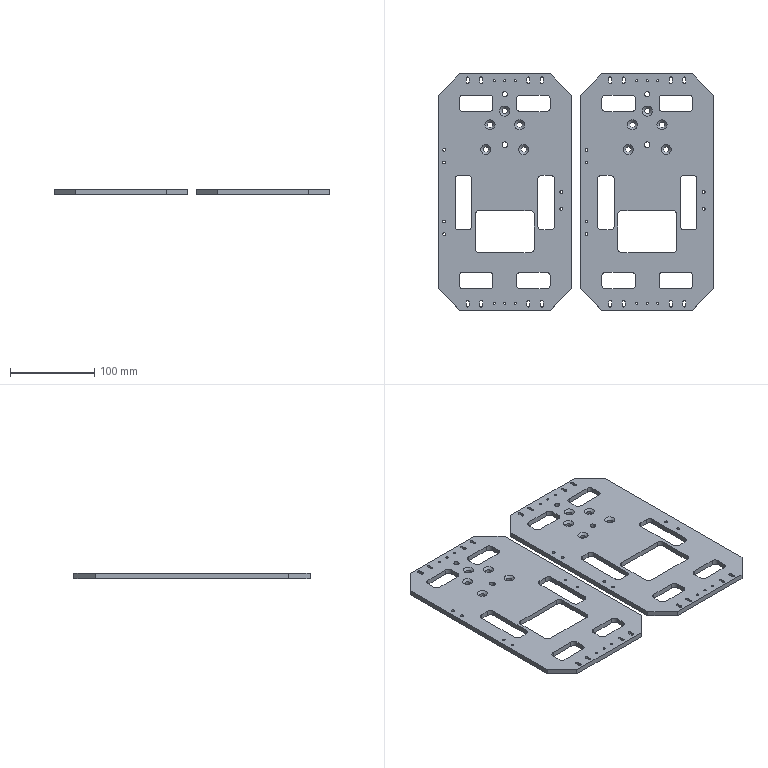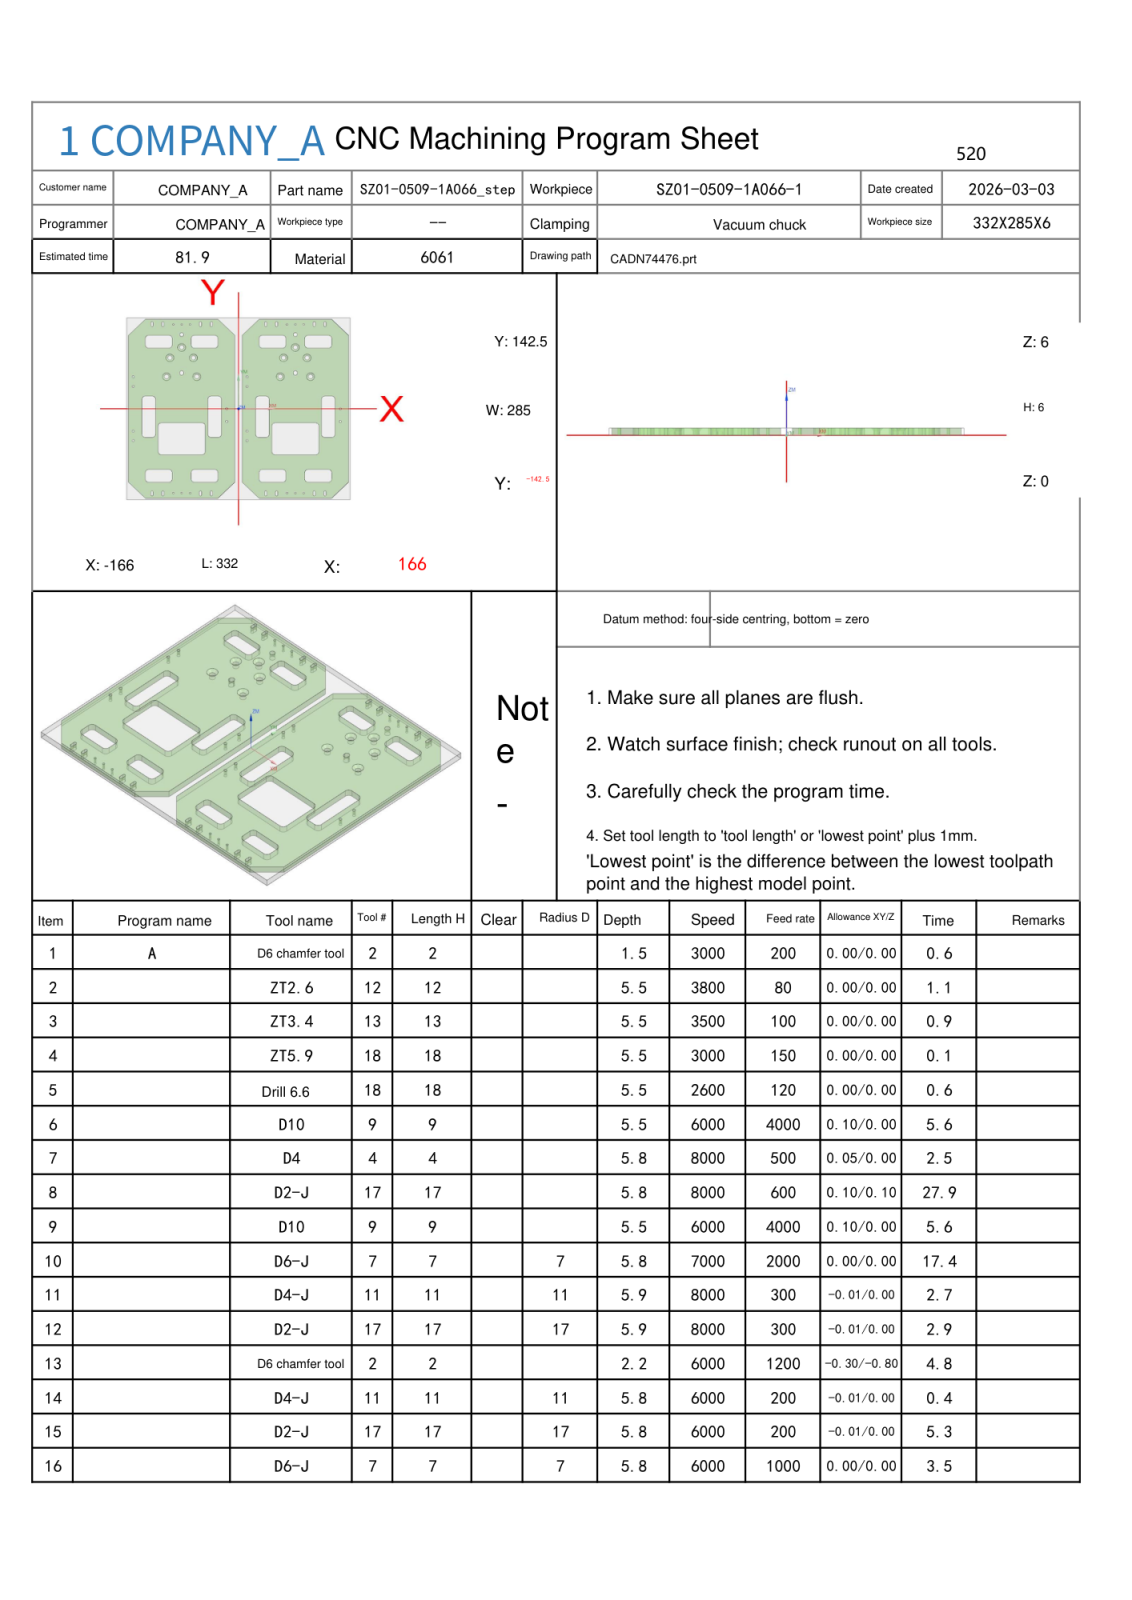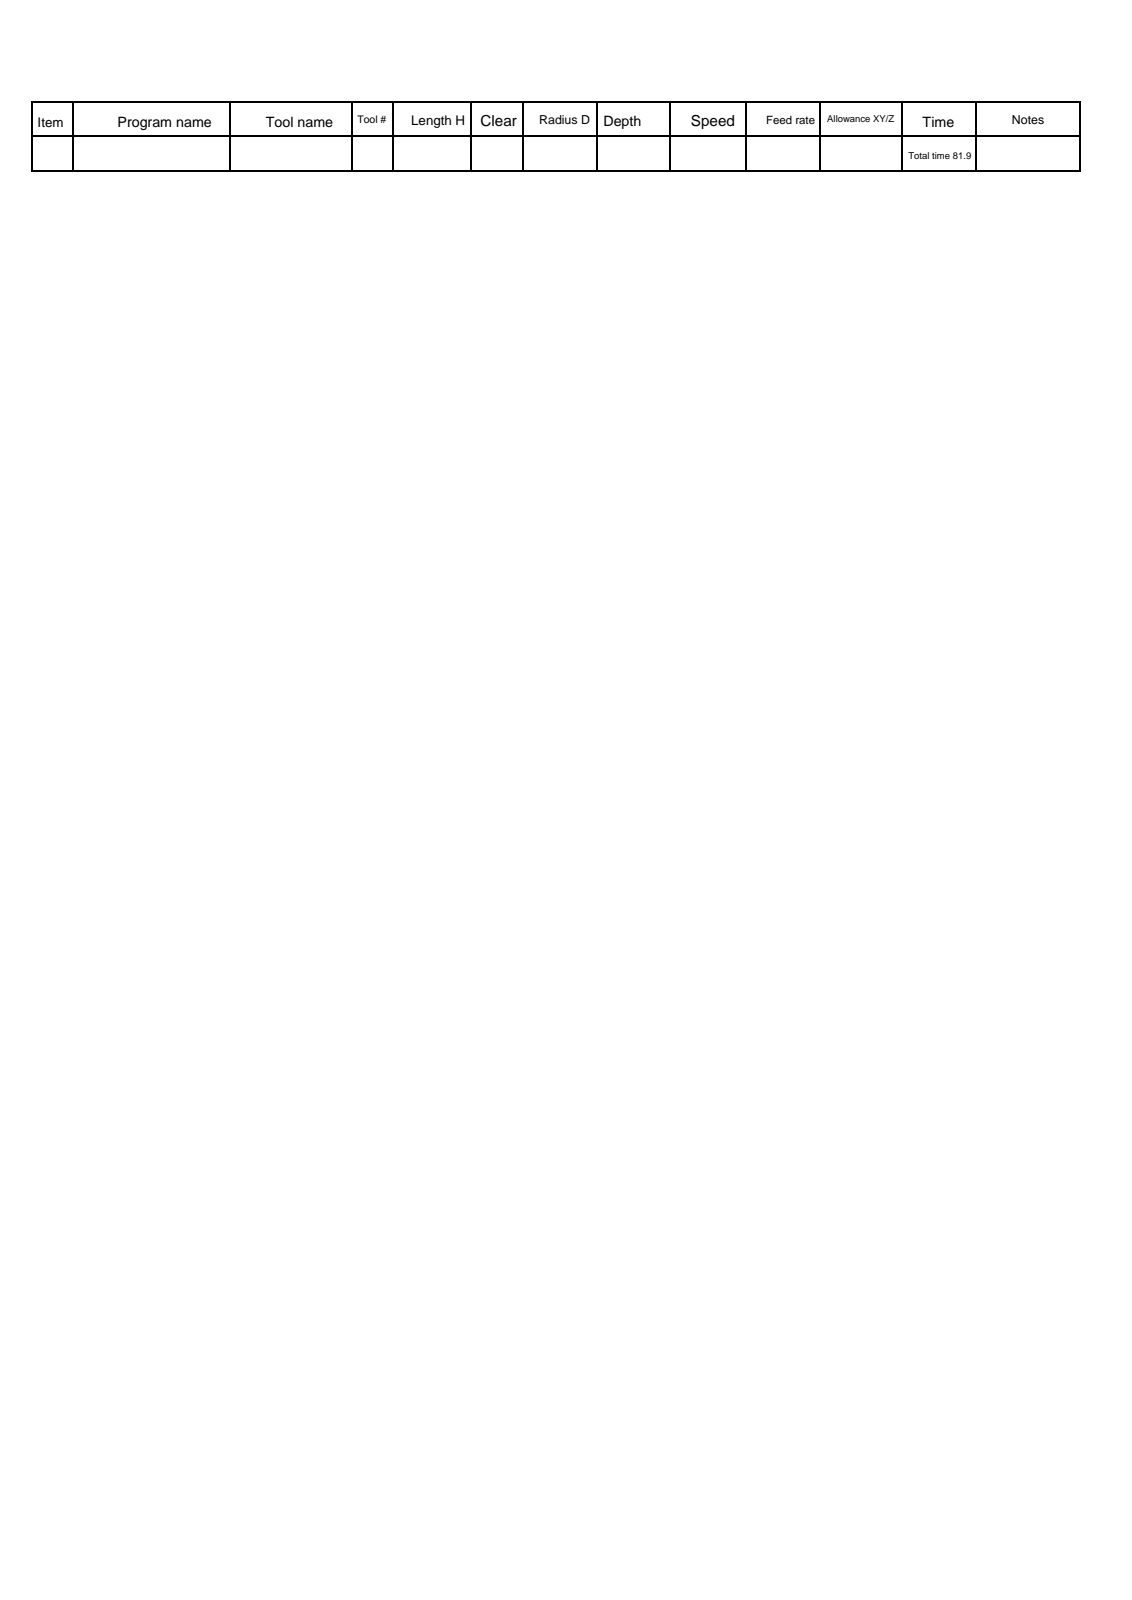NC program | NX | posted by the shop | part box 327 x 280 x 6 mm
Lines 10363 to 11471 of 31860:
N10 T07 M06
(D6-J  D=6. R=0. H=07 ce=0.00 di=0.00)
G00 G90 G54 X53.5 Y-66.801 M03 S6000
G43 H07 Z36.
M08
Z1.
G01 Z.5 F1000.
G41 D07
Y-68.
G03 X54.5 Y-69. I1. J0.0
G01 X114.5
G03 X116.5 Y-67. I0.0 J2.
G01 Y-27.
G03 X114.5 Y-25. I-2. J0.0
G01 X54.5
G03 X52.5 Y-27. I0.0 J-2.
G01 Y-67.
G03 X54.5 Y-69. I2. J0.0
G01 X55.
G03 X56. Y-68. I0.0 J1.
G01 G40 Y-67.8
Z1.
G00 Z36.
X-115.5 Y-66.801
Z1.
G01 Z.5
G41 D07
Y-68.
G03 X-114.5 Y-69. I1. J0.0
G01 X-54.5
G03 X-52.5 Y-67. I0.0 J2.
G01 Y-27.
G03 X-54.5 Y-25. I-2. J0.0
G01 X-114.5
G03 X-116.5 Y-27. I0.0 J-2.
G01 Y-67.
G03 X-114.5 Y-69. I2. J0.0
G01 X-114.
G03 X-113. Y-68. I0.0 J1.
G01 G40 Y-67.8
Z1.
G00 Z36.
G00 G90 X138.3 Y-41. M03 S6000
Z36.
Z1.
G01 Z.5 F1000.
G41 D07
X139.5
G03 X140.5 Y-40. I0.0 J1.
G01 Y15.
G03 X138.5 Y17. I-2. J0.0
G01 X128.5
G03 X126.5 Y15. I0.0 J-2.
G01 Y-40.
G03 X128.5 Y-42. I2. J0.0
G01 X138.5
G03 X140.5 Y-40. I0.0 J2.
G01 Y-39.5
G03 X139.5 Y-38.5 I-1. J0.0
G01 G40 X139.3
Z1.
G00 Z36.
X40.301 Y-41.
Z1.
G01 Z.5
G41 D07
X41.5
G03 X42.5 Y-40. I0.0 J1.
G01 Y15.
G03 X40.5 Y17. I-2. J0.0
G01 X30.5
G03 X28.5 Y15. I0.0 J-2.
G01 Y-40.
G03 X30.5 Y-42. I2. J0.0
G01 X40.5
G03 X42.5 Y-40. I0.0 J2.
G01 Y-39.5
G03 X41.5 Y-38.5 I-1. J0.0
G01 G40 X41.3
Z1.
G00 Z36.
X-40.301 Y16.
Z1.
G01 Z.5
G41 D07
X-41.5
G03 X-42.5 Y15. I0.0 J-1.
G01 Y-40.
G03 X-40.5 Y-42. I2. J0.0
G01 X-30.5
G03 X-28.5 Y-40. I0.0 J2.
G01 Y15.
G03 X-30.5 Y17. I-2. J0.0
G01 X-40.5
G03 X-42.5 Y15. I0.0 J-2.
G01 Y14.5
G03 X-41.5 Y13.5 I1. J0.0
G01 G40 X-41.3
Z1.
G00 Z36.
X-138.301 Y16.
Z1.
G01 Z.5
G41 D07
X-139.5
G03 X-140.5 Y15. I0.0 J-1.
G01 Y-40.
G03 X-138.5 Y-42. I2. J0.0
G01 X-128.5
G03 X-126.5 Y-40. I0.0 J2.
G01 Y15.
G03 X-128.5 Y17. I-2. J0.0
G01 X-138.5
G03 X-140.5 Y15. I0.0 J-2.
G01 Y14.5
G03 X-139.5 Y13.5 I1. J0.0
G01 G40 X-139.3
Z1.
G00 Z36.
G00 G90 X-102.5 Y109.8 M03 S6000
Z36.
Z1.
G01 Z.5 F1000.
G41 D07
Y111.
G03 X-103.5 Y112. I-1. J0.0
G01 X-133.5
G03 X-135.5 Y110. I0.0 J-2.
G01 Y100.
G03 X-133.5 Y98. I2. J0.0
G01 X-103.5
G03 X-101.5 Y100. I0.0 J2.
G01 Y110.
G03 X-103.5 Y112. I-2. J0.0
G01 X-104.
G03 X-105. Y111. I0.0 J-1.
G01 G40 Y110.8
Z1.
G00 Z36.
X-34.5 Y109.8
Z1.
G01 Z.5
G41 D07
Y111.
G03 X-35.5 Y112. I-1. J0.0
G01 X-65.5
G03 X-67.5 Y110. I0.0 J-2.
G01 Y100.
G03 X-65.5 Y98. I2. J0.0
G01 X-35.5
G03 X-33.5 Y100. I0.0 J2.
G01 Y110.
G03 X-35.5 Y112. I-2. J0.0
G01 X-36.
G03 X-37. Y111. I0.0 J-1.
G01 G40 Y110.8
Z1.
G00 Z36.
X66.5 Y109.8
Z1.
G01 Z.5
G41 D07
Y111.
G03 X65.5 Y112. I-1. J0.0
G01 X35.5
G03 X33.5 Y110. I0.0 J-2.
G01 Y100.
G03 X35.5 Y98. I2. J0.0
G01 X65.5
G03 X67.5 Y100. I0.0 J2.
G01 Y110.
G03 X65.5 Y112. I-2. J0.0
G01 X65.
G03 X64. Y111. I0.0 J-1.
G01 G40 Y110.8
Z1.
G00 Z36.
X134.5 Y109.8
Z1.
G01 Z.5
G41 D07
Y111.
G03 X133.5 Y112. I-1. J0.0
G01 X103.5
G03 X101.5 Y110. I0.0 J-2.
G01 Y100.
G03 X103.5 Y98. I2. J0.0
G01 X133.5
G03 X135.5 Y100. I0.0 J2.
G01 Y110.
G03 X133.5 Y112. I-2. J0.0
G01 X133.
G03 X132. Y111. I0.0 J-1.
G01 G40 Y110.8
Z1.
G00 Z36.
X102.5 Y-109.8
Z1.
G01 Z.5
G41 D07
Y-111.
G03 X103.5 Y-112. I1. J0.0
G01 X133.5
G03 X135.5 Y-110. I0.0 J2.
G01 Y-100.
G03 X133.5 Y-98. I-2. J0.0
G01 X103.5
G03 X101.5 Y-100. I0.0 J-2.
G01 Y-110.
G03 X103.5 Y-112. I2. J0.0
G01 X104.
G03 X105. Y-111. I0.0 J1.
G01 G40 Y-110.8
Z1.
G00 Z36.
X34.793 Y-110.707
Z1.
G01 Z.5
G41 D07
X34.5 Y-111.
G03 X35.5 Y-112. I1. J0.0
G01 X65.5
G03 X67.5 Y-110. I0.0 J2.
G01 Y-100.
G03 X65.5 Y-98. I-2. J0.0
G01 X35.5
G03 X33.5 Y-100. I0.0 J-2.
G01 Y-110.
G03 X35.5 Y-112. I2. J0.0
G01 X36.
G03 X37. Y-111. I0.0 J1.
G01 G40 Y-110.8
Z1.
G00 Z36.
X-66.5 Y-109.8
Z1.
G01 Z.5
G41 D07
Y-111.
G03 X-65.5 Y-112. I1. J0.0
G01 X-35.5
G03 X-33.5 Y-110. I0.0 J2.
G01 Y-100.
G03 X-35.5 Y-98. I-2. J0.0
G01 X-65.5
G03 X-67.5 Y-100. I0.0 J-2.
G01 Y-110.
G03 X-65.5 Y-112. I2. J0.0
G01 X-65.
G03 X-64. Y-111. I0.0 J1.
G01 G40 Y-110.8
Z1.
G00 Z36.
X-134.5 Y-109.8
Z1.
G01 Z.5
G41 D07
Y-111.
G03 X-133.5 Y-112. I1. J0.0
G01 X-103.5
G03 X-101.5 Y-110. I0.0 J2.
G01 Y-100.
G03 X-103.5 Y-98. I-2. J0.0
G01 X-133.5
G03 X-135.5 Y-100. I0.0 J-2.
G01 Y-110.
G03 X-133.5 Y-112. I2. J0.0
G01 X-133.
G03 X-132. Y-111. I0.0 J1.
G01 G40 Y-110.8
Z1.
G00 Z36.
G00 G90 X53.5 Y-66.901 M03 S6000
Z36.
Z.7
G01 Z.2 F1000.
G41 D07
Y-68.
G03 X54.5 Y-69. I1. J0.0
G01 X114.5
G03 X116.5 Y-67. I0.0 J2.
G01 Y-27.
G03 X114.5 Y-25. I-2. J0.0
G01 X54.5
G03 X52.5 Y-27. I0.0 J-2.
G01 Y-67.
G03 X54.5 Y-69. I2. J0.0
G01 X55.
G03 X56. Y-68. I0.0 J1.
G01 G40 Y-67.9
Z.7
G00 Z36.
X-115.5 Y-66.9
Z.7
G01 Z.2
G41 D07
Y-68.
G03 X-114.5 Y-69. I1. J0.0
G01 X-54.5
G03 X-52.5 Y-67. I0.0 J2.
G01 Y-27.
G03 X-54.5 Y-25. I-2. J0.0
G01 X-114.5
G03 X-116.5 Y-27. I0.0 J-2.
G01 Y-67.
G03 X-114.5 Y-69. I2. J0.0
G01 X-114.
G03 X-113. Y-68. I0.0 J1.
G01 G40 Y-67.9
Z.7
G00 Z36.
G00 G90 X138.401 Y-41. M03 S6000
Z36.
Z.7
G01 Z.2 F1000.
G41 D07
X139.5
G03 X140.5 Y-40. I0.0 J1.
G01 Y15.
G03 X138.5 Y17. I-2. J0.0
G01 X128.5
G03 X126.5 Y15. I0.0 J-2.
G01 Y-40.
G03 X128.5 Y-42. I2. J0.0
G01 X138.5
G03 X140.5 Y-40. I0.0 J2.
G01 Y-39.5
G03 X139.5 Y-38.5 I-1. J0.0
G01 G40 X139.4
Z.7
G00 Z36.
X40.4 Y-41.
Z.7
G01 Z.2
G41 D07
X41.5
G03 X42.5 Y-40. I0.0 J1.
G01 Y15.
G03 X40.5 Y17. I-2. J0.0
G01 X30.5
G03 X28.5 Y15. I0.0 J-2.
G01 Y-40.
G03 X30.5 Y-42. I2. J0.0
G01 X40.5
G03 X42.5 Y-40. I0.0 J2.
G01 Y-39.5
G03 X41.5 Y-38.5 I-1. J0.0
G01 G40 X41.4
Z.7
G00 Z36.
X-40.401 Y16.
Z.7
G01 Z.2
G41 D07
X-41.5
G03 X-42.5 Y15. I0.0 J-1.
G01 Y-40.
G03 X-40.5 Y-42. I2. J0.0
G01 X-30.5
G03 X-28.5 Y-40. I0.0 J2.
G01 Y15.
G03 X-30.5 Y17. I-2. J0.0
G01 X-40.5
G03 X-42.5 Y15. I0.0 J-2.
G01 Y14.5
G03 X-41.5 Y13.5 I1. J0.0
G01 G40 X-41.4
Z.7
G00 Z36.
X-138.4 Y16.
Z.7
G01 Z.2
G41 D07
X-139.5
G03 X-140.5 Y15. I0.0 J-1.
G01 Y-40.
G03 X-138.5 Y-42. I2. J0.0
G01 X-128.5
G03 X-126.5 Y-40. I0.0 J2.
G01 Y15.
G03 X-128.5 Y17. I-2. J0.0
G01 X-138.5
G03 X-140.5 Y15. I0.0 J-2.
G01 Y14.5
G03 X-139.5 Y13.5 I1. J0.0
G01 G40 X-139.4
Z.7
G00 Z36.
G00 G90 X-102.793 Y110.707 M03 S6000
Z36.
Z.7
G01 Z.2 F1000.
G41 D07
X-102.5 Y111.
G03 X-103.5 Y112. I-1. J0.0
G01 X-133.5
G03 X-135.5 Y110. I0.0 J-2.
G01 Y100.
G03 X-133.5 Y98. I2. J0.0
G01 X-103.5
G03 X-101.5 Y100. I0.0 J2.
G01 Y110.
G03 X-103.5 Y112. I-2. J0.0
G01 X-104.
G03 X-105. Y111. I0.0 J-1.
G01 G40 Y110.9
Z.7
G00 Z36.
X-34.5 Y109.9
Z.7
G01 Z.2
G41 D07
Y111.
G03 X-35.5 Y112. I-1. J0.0
G01 X-65.5
G03 X-67.5 Y110. I0.0 J-2.
G01 Y100.
G03 X-65.5 Y98. I2. J0.0
G01 X-35.5
G03 X-33.5 Y100. I0.0 J2.
G01 Y110.
G03 X-35.5 Y112. I-2. J0.0
G01 X-36.
G03 X-37. Y111. I0.0 J-1.
G01 G40 Y110.9
Z.7
G00 Z36.
X66.5 Y109.9
Z.7
G01 Z.2
G41 D07
Y111.
G03 X65.5 Y112. I-1. J0.0
G01 X35.5
G03 X33.5 Y110. I0.0 J-2.
G01 Y100.
G03 X35.5 Y98. I2. J0.0
G01 X65.5
G03 X67.5 Y100. I0.0 J2.
G01 Y110.
G03 X65.5 Y112. I-2. J0.0
G01 X65.
G03 X64. Y111. I0.0 J-1.
G01 G40 Y110.9
Z.7
G00 Z36.
X134.5 Y109.9
Z.7
G01 Z.2
G41 D07
Y111.
G03 X133.5 Y112. I-1. J0.0
G01 X103.5
G03 X101.5 Y110. I0.0 J-2.
G01 Y100.
G03 X103.5 Y98. I2. J0.0
G01 X133.5
G03 X135.5 Y100. I0.0 J2.
G01 Y110.
G03 X133.5 Y112. I-2. J0.0
G01 X133.
G03 X132. Y111. I0.0 J-1.
G01 G40 Y110.9
Z.7
G00 Z36.
X102.5 Y-109.9
Z.7
G01 Z.2
G41 D07
Y-111.
G03 X103.5 Y-112. I1. J0.0
G01 X133.5
G03 X135.5 Y-110. I0.0 J2.
G01 Y-100.
G03 X133.5 Y-98. I-2. J0.0
G01 X103.5
G03 X101.5 Y-100. I0.0 J-2.
G01 Y-110.
G03 X103.5 Y-112. I2. J0.0
G01 X104.
G03 X105. Y-111. I0.0 J1.
G01 G40 Y-110.9
Z.7
G00 Z36.
X34.5 Y-109.901
Z.7
G01 Z.2
G41 D07
Y-111.
G03 X35.5 Y-112. I1. J0.0
G01 X65.5
G03 X67.5 Y-110. I0.0 J2.
G01 Y-100.
G03 X65.5 Y-98. I-2. J0.0
G01 X35.5
G03 X33.5 Y-100. I0.0 J-2.
G01 Y-110.
G03 X35.5 Y-112. I2. J0.0
G01 X36.
G03 X37. Y-111. I0.0 J1.
G01 G40 Y-110.9
Z.7
G00 Z36.
X-66.5 Y-109.9
Z.7
G01 Z.2
G41 D07
Y-111.
G03 X-65.5 Y-112. I1. J0.0
G01 X-35.5
G03 X-33.5 Y-110. I0.0 J2.
G01 Y-100.
G03 X-35.5 Y-98. I-2. J0.0
G01 X-65.5
G03 X-67.5 Y-100. I0.0 J-2.
G01 Y-110.
G03 X-65.5 Y-112. I2. J0.0
G01 X-65.
G03 X-64. Y-111. I0.0 J1.
G01 G40 Y-110.9
Z.7
G00 Z36.
X-134.5 Y-109.9
Z.7
G01 Z.2
G41 D07
Y-111.
G03 X-133.5 Y-112. I1. J0.0
G01 X-103.5
G03 X-101.5 Y-110. I0.0 J2.
G01 Y-100.
G03 X-103.5 Y-98. I-2. J0.0
G01 X-133.5
G03 X-135.5 Y-100. I0.0 J-2.
G01 Y-110.
G03 X-133.5 Y-112. I2. J0.0
G01 X-133.
G03 X-132. Y-111. I0.0 J1.
G01 G40 Y-110.9
Z.7
G00 Z36.
G00 G90 X-104.104 Y49.533 M03 S7000
Z36.
Z7.5
G01 X-104.1 Y49.546 Z7.499 F2000.
X-104.025 Y50.008 Z7.475
X-104.024 Y50.476 Z7.45
X-104.096 Y50.938 Z7.426
X-104.239 Y51.384 Z7.401
X-104.45 Y51.801 Z7.377
X-104.724 Y52.181 Z7.352
X-105.054 Y52.513 Z7.328
X-105.431 Y52.789 Z7.303
X-105.848 Y53.003 Z7.279
X-106.292 Y53.149 Z7.254
X-106.632 Y53.212 Z7.236
X-107.072 Y53.234 Z7.213
X-107.416 Y53.205 Z7.195
X-107.861 Y53.108 Z7.171
X-108.285 Y52.944 Z7.147
X-108.679 Y52.717 Z7.123
X-109.035 Y52.433 Z7.099
X-109.343 Y52.099 Z7.076
X-109.596 Y51.721 Z7.052
X-109.79 Y51.31 Z7.028
X-109.919 Y50.873 Z7.004
X-109.979 Y50.423 Z6.98
Y50.077 Z6.962
X-109.93 Y49.684 Z6.941
X-109.83 Y49.301 Z6.921
X-109.679 Y48.935 Z6.9
X-109.509 Y48.634 Z6.882
X-109.223 Y48.259 Z6.857
X-108.881 Y47.933 Z6.832
X-108.492 Y47.665 Z6.807
X-108.065 Y47.462 Z6.783
X-107.612 Y47.329 Z6.758
X-107.143 Y47.269 Z6.733
X-106.671 Y47.284 Z6.708
X-106.207 Y47.373 Z6.684
X-105.763 Y47.534 Z6.659
X-105.35 Y47.763 Z6.634
X-104.978 Y48.055 Z6.609
X-104.657 Y48.402 Z6.585
X-104.459 Y48.685 Z6.567
X-104.246 Y49.101 Z6.542
X-104.1 Y49.546 Z6.518
X-104.025 Y50.008 Z6.493
X-104.024 Y50.476 Z6.468
X-104.096 Y50.938 Z6.444
X-104.239 Y51.384 Z6.419
X-104.45 Y51.801 Z6.395
X-104.724 Y52.181 Z6.37
X-105.054 Y52.513 Z6.346
X-105.431 Y52.789 Z6.321
X-105.848 Y53.003 Z6.297
X-106.292 Y53.149 Z6.272
X-106.632 Y53.212 Z6.254
X-107.072 Y53.234 Z6.231
X-107.416 Y53.205 Z6.213
X-107.861 Y53.108 Z6.189
X-108.285 Y52.944 Z6.165
X-108.679 Y52.717 Z6.141
X-109.035 Y52.433 Z6.118
X-109.343 Y52.099 Z6.094
X-109.596 Y51.721 Z6.07
X-109.79 Y51.31 Z6.046
X-109.919 Y50.873 Z6.022
X-109.979 Y50.423 Z5.998
Y50.25 Z5.989
G03 X-107. Y47.271 I2.979 J0.0
X-104.021 Y50.25 I0.0 J2.979
X-107. Y53.229 I-2.979 J0.0
X-109.979 Y50.25 I0.0 J-2.979
G01 X-109.973 Y50.19 Z5.984
X-109.966 Y50.129 Z5.979
G03 X-107. Y47.281 I2.966 J.121
X-104.031 Y50.25 I0.0 J2.969
X-107. Y53.219 I-2.969 J0.0
X-109.969 Y50.25 I0.0 J-2.969
G01 X-109.963 Y50.19 Z5.973
X-109.956 Y50.129 Z5.968
G03 X-107. Y47.292 I2.956 J.121
X-104.042 Y50.25 I0.0 J2.958
X-107. Y53.208 I-2.958 J0.0
X-109.958 Y50.25 I0.0 J-2.958
G01 X-109.952 Y50.19 Z5.963
X-109.945 Y50.129 Z5.958
G03 X-107. Y47.302 I2.945 J.121
X-104.052 Y50.25 I0.0 J2.948
X-107. Y53.198 I-2.948 J0.0
X-109.948 Y50.25 I0.0 J-2.948
G01 X-109.942 Y50.19 Z5.952
X-109.934 Y50.129 Z5.947
G03 X-107. Y47.313 I2.934 J.121
X-104.063 Y50.25 I0.0 J2.937
X-107. Y53.187 I-2.937 J0.0
X-109.937 Y50.25 I0.0 J-2.937
G01 X-109.931 Y50.19 Z5.942
X-109.924 Y50.129 Z5.936
G03 X-107. Y47.324 I2.924 J.121
X-104.074 Y50.25 I0.0 J2.926
X-107. Y53.176 I-2.926 J0.0
X-109.926 Y50.25 I0.0 J-2.926
G01 X-109.92 Y50.19 Z5.931
X-109.913 Y50.129 Z5.926
G03 X-107. Y47.334 I2.913 J.121
X-104.084 Y50.25 I0.0 J2.916
X-107. Y53.166 I-2.916 J0.0
X-109.916 Y50.25 I0.0 J-2.916
G01 X-109.91 Y50.19 Z5.92
X-109.903 Y50.129 Z5.915
G03 X-107. Y47.345 I2.903 J.121
X-104.095 Y50.25 I0.0 J2.905
X-107. Y53.155 I-2.905 J0.0
X-109.905 Y50.25 I0.0 J-2.905
G01 X-109.899 Y50.19 Z5.91
X-109.892 Y50.129 Z5.905
G03 X-107. Y47.355 I2.892 J.121
X-104.105 Y50.25 I0.0 J2.895
X-107. Y53.145 I-2.895 J0.0
X-109.895 Y50.25 I0.0 J-2.895
G01 X-109.889 Y50.19 Z5.899
X-109.881 Y50.129 Z5.894
G03 X-107. Y47.366 I2.881 J.121
X-104.116 Y50.25 I0.0 J2.884
X-107. Y53.134 I-2.884 J0.0
X-109.884 Y50.25 I0.0 J-2.884
G01 X-109.878 Y50.19 Z5.889
X-109.871 Y50.129 Z5.883
G03 X-107. Y47.377 I2.871 J.121
X-104.127 Y50.25 I0.0 J2.873
X-107. Y53.123 I-2.873 J0.0
X-109.873 Y50.25 I0.0 J-2.873
G01 X-109.867 Y50.19 Z5.878
X-109.86 Y50.129 Z5.873
G03 X-107. Y47.387 I2.86 J.121
X-104.137 Y50.25 I0.0 J2.863
X-107. Y53.113 I-2.863 J0.0
X-109.863 Y50.25 I0.0 J-2.863
G01 X-109.857 Y50.19 Z5.867
X-109.85 Y50.129 Z5.862
G03 X-107. Y47.398 I2.85 J.121
X-104.148 Y50.25 I0.0 J2.852
X-107. Y53.102 I-2.852 J0.0
X-109.852 Y50.25 I0.0 J-2.852
G01 X-109.846 Y50.19 Z5.857
X-109.839 Y50.129 Z5.852
G03 X-107. Y47.408 I2.839 J.121
X-104.158 Y50.25 I0.0 J2.842
X-107. Y53.092 I-2.842 J0.0
X-109.842 Y50.25 I0.0 J-2.842
G01 X-109.836 Y50.19 Z5.846
X-109.828 Y50.129 Z5.841
G03 X-107. Y47.419 I2.828 J.121
X-104.169 Y50.25 I0.0 J2.831
X-107. Y53.081 I-2.831 J0.0
X-109.831 Y50.25 I0.0 J-2.831
G01 X-109.825 Y50.19 Z5.836
X-109.818 Y50.129 Z5.83
G03 X-107. Y47.43 I2.818 J.121
X-104.18 Y50.25 I0.0 J2.82
X-107. Y53.07 I-2.82 J0.0
X-109.82 Y50.25 I0.0 J-2.82
G01 X-109.814 Y50.19 Z5.825
X-109.807 Y50.129 Z5.82
G03 X-107. Y47.44 I2.807 J.121
X-104.19 Y50.25 I0.0 J2.81
X-107. Y53.06 I-2.81 J0.0
X-109.81 Y50.25 I0.0 J-2.81
G01 X-109.804 Y50.19 Z5.814
X-109.796 Y50.129 Z5.809
G03 X-107. Y47.451 I2.796 J.121
X-104.201 Y50.25 I0.0 J2.799
X-107. Y53.049 I-2.799 J0.0
X-109.799 Y50.25 I0.0 J-2.799
G01 X-109.793 Y50.19 Z5.804
X-109.786 Y50.129 Z5.798
G03 X-107. Y47.462 I2.786 J.121
X-104.212 Y50.25 I0.0 J2.788
X-107. Y53.038 I-2.788 J0.0
X-109.788 Y50.25 I0.0 J-2.788
G01 X-109.783 Y50.19 Z5.793
X-109.775 Y50.129 Z5.788
G03 X-107. Y47.472 I2.775 J.121
X-104.222 Y50.25 I0.0 J2.778
X-107. Y53.028 I-2.778 J0.0
X-109.778 Y50.25 I0.0 J-2.778
G01 X-109.772 Y50.19 Z5.783
X-109.765 Y50.129 Z5.777
G03 X-107. Y47.483 I2.765 J.121
X-104.233 Y50.25 I0.0 J2.767
X-107. Y53.017 I-2.767 J0.0
X-109.767 Y50.25 I0.0 J-2.767
G01 X-109.761 Y50.19 Z5.772
X-109.754 Y50.129 Z5.767
G03 X-107. Y47.493 I2.754 J.121
X-104.243 Y50.25 I0.0 J2.757
X-107. Y53.007 I-2.757 J0.0
X-109.757 Y50.25 I0.0 J-2.757
G01 X-109.751 Y50.19 Z5.761
X-109.743 Y50.129 Z5.756
G03 X-107. Y47.504 I2.743 J.121
X-104.254 Y50.25 I0.0 J2.746
X-107. Y52.996 I-2.746 J0.0
X-109.746 Y50.25 I0.0 J-2.746
G01 X-109.74 Y50.19 Z5.751
X-109.733 Y50.129 Z5.745
G03 X-107. Y47.515 I2.733 J.121
X-104.265 Y50.25 I0.0 J2.735
X-107. Y52.985 I-2.735 J0.0
X-109.735 Y50.25 I0.0 J-2.735
G01 X-109.729 Y50.19 Z5.74
X-109.722 Y50.129 Z5.735
G03 X-107. Y47.525 I2.722 J.121
X-104.275 Y50.25 I0.0 J2.725
X-107. Y52.975 I-2.725 J0.0
X-109.725 Y50.25 I0.0 J-2.725
G01 X-109.719 Y50.19 Z5.73
X-109.712 Y50.129 Z5.724
G03 X-107. Y47.536 I2.712 J.121
X-104.286 Y50.25 I0.0 J2.714
X-107. Y52.964 I-2.714 J0.0
X-109.714 Y50.25 I0.0 J-2.714
G01 X-109.708 Y50.19 Z5.719
X-109.701 Y50.129 Z5.714
G03 X-107. Y47.546 I2.701 J.121
X-104.296 Y50.25 I0.0 J2.704
X-107. Y52.954 I-2.704 J0.0
X-109.704 Y50.25 I0.0 J-2.704
G01 X-109.698 Y50.19 Z5.708
X-109.69 Y50.129 Z5.703
G03 X-107. Y47.557 I2.69 J.121
X-104.307 Y50.25 I0.0 J2.693
X-107. Y52.943 I-2.693 J0.0
X-109.693 Y50.25 I0.0 J-2.693
G01 X-109.687 Y50.19 Z5.698
X-109.68 Y50.129 Z5.692
G03 X-107. Y47.568 I2.68 J.121
X-104.318 Y50.25 I0.0 J2.682
X-107. Y52.932 I-2.682 J0.0
X-109.682 Y50.25 I0.0 J-2.682
G01 X-109.676 Y50.19 Z5.687
X-109.669 Y50.129 Z5.682
G03 X-107. Y47.578 I2.669 J.121
X-104.328 Y50.25 I0.0 J2.672
X-107. Y52.922 I-2.672 J0.0
X-109.672 Y50.25 I0.0 J-2.672
G01 X-109.666 Y50.19 Z5.676
X-109.658 Y50.129 Z5.671
G03 X-107. Y47.589 I2.658 J.121
X-104.339 Y50.25 I0.0 J2.661
X-107. Y52.911 I-2.661 J0.0
X-109.661 Y50.25 I0.0 J-2.661
G01 X-109.655 Y50.19 Z5.666
X-109.648 Y50.129 Z5.661
G03 X-107. Y47.599 I2.648 J.121
X-104.349 Y50.25 I0.0 J2.651
X-107. Y52.901 I-2.651 J0.0
X-109.651 Y50.25 I0.0 J-2.651
G01 X-109.645 Y50.19 Z5.655
X-109.637 Y50.129 Z5.65
G03 X-107. Y47.61 I2.637 J.121
X-104.36 Y50.25 I0.0 J2.64
X-107. Y52.89 I-2.64 J0.0
X-109.64 Y50.25 I0.0 J-2.64
G01 X-109.634 Y50.19 Z5.645
X-109.627 Y50.129 Z5.639
G03 X-107. Y47.621 I2.627 J.121
X-104.371 Y50.25 I0.0 J2.629
X-107. Y52.879 I-2.629 J0.0
X-109.629 Y50.25 I0.0 J-2.629
G01 X-109.623 Y50.19 Z5.634
X-109.616 Y50.129 Z5.629
G03 X-107. Y47.631 I2.616 J.121
X-104.381 Y50.25 I0.0 J2.619
X-107. Y52.869 I-2.619 J0.0
X-109.619 Y50.25 I0.0 J-2.619
G01 X-109.613 Y50.19 Z5.623
X-109.605 Y50.129 Z5.618
G03 X-107. Y47.642 I2.605 J.121
X-104.392 Y50.25 I0.0 J2.608
X-107. Y52.858 I-2.608 J0.0
X-109.608 Y50.25 I0.0 J-2.608
G01 X-109.602 Y50.19 Z5.613
X-109.595 Y50.129 Z5.608
G03 X-107. Y47.652 I2.595 J.121
X-104.402 Y50.25 I0.0 J2.598
X-107. Y52.848 I-2.598 J0.0
X-109.598 Y50.25 I0.0 J-2.598
G01 X-109.592 Y50.19 Z5.602
X-109.584 Y50.129 Z5.597
G03 X-107. Y47.663 I2.584 J.121
X-104.413 Y50.25 I0.0 J2.587
X-107. Y52.837 I-2.587 J0.0
X-109.587 Y50.25 I0.0 J-2.587
G01 X-109.581 Y50.19 Z5.592
X-109.574 Y50.129 Z5.586
G03 X-107. Y47.674 I2.574 J.121
X-104.424 Y50.25 I0.0 J2.576
X-107. Y52.826 I-2.576 J0.0
X-109.576 Y50.25 I0.0 J-2.576
G01 X-109.57 Y50.19 Z5.581
X-109.563 Y50.129 Z5.576
G03 X-107. Y47.684 I2.563 J.121
X-104.434 Y50.25 I0.0 J2.566
X-107. Y52.816 I-2.566 J0.0
X-109.566 Y50.25 I0.0 J-2.566
G01 X-109.56 Y50.19 Z5.57
X-109.552 Y50.129 Z5.565
G03 X-107. Y47.695 I2.552 J.121
X-104.445 Y50.25 I0.0 J2.555
X-107. Y52.805 I-2.555 J0.0
X-109.555 Y50.25 I0.0 J-2.555
G01 X-109.549 Y50.19 Z5.56
X-109.542 Y50.129 Z5.555
G03 X-107. Y47.705 I2.542 J.121
X-104.455 Y50.25 I0.0 J2.545
X-107. Y52.795 I-2.545 J0.0
X-109.545 Y50.25 I0.0 J-2.545
G01 X-109.539 Y50.19 Z5.549
X-109.531 Y50.129 Z5.544
G03 X-107. Y47.716 I2.531 J.121
X-104.466 Y50.25 I0.0 J2.534
X-107. Y52.784 I-2.534 J0.0
X-109.534 Y50.25 I0.0 J-2.534
G01 X-109.528 Y50.19 Z5.539
X-109.52 Y50.129 Z5.533
G03 X-107. Y47.727 I2.52 J.121
X-104.477 Y50.25 I0.0 J2.523
X-107. Y52.773 I-2.523 J0.0
X-109.523 Y50.25 I0.0 J-2.523
G01 X-109.517 Y50.19 Z5.528
X-109.51 Y50.129 Z5.523
G03 X-107. Y47.737 I2.51 J.121
X-104.487 Y50.25 I0.0 J2.513
X-107. Y52.763 I-2.513 J0.0
X-109.513 Y50.25 I0.0 J-2.513
G01 X-109.507 Y50.19 Z5.517
X-109.499 Y50.129 Z5.512
G03 X-107. Y47.748 I2.499 J.121
X-104.498 Y50.25 I0.0 J2.502
X-107. Y52.752 I-2.502 J0.0
X-109.502 Y50.25 I0.0 J-2.502
G01 X-109.496 Y50.19 Z5.507
X-109.489 Y50.129 Z5.501
G03 X-107. Y47.759 I2.489 J.121
X-104.509 Y50.25 I0.0 J2.491
X-107. Y52.741 I-2.491 J0.0
X-109.491 Y50.25 I0.0 J-2.491
G01 X-109.485 Y50.19 Z5.496
X-109.478 Y50.129 Z5.491
G03 X-107. Y47.769 I2.478 J.121
X-104.519 Y50.25 I0.0 J2.481
X-107. Y52.731 I-2.481 J0.0
X-109.481 Y50.25 I0.0 J-2.481
G01 X-109.475 Y50.19 Z5.486
X-109.467 Y50.129 Z5.48
G03 X-107. Y47.78 I2.467 J.121
X-104.53 Y50.25 I0.0 J2.47
X-107. Y52.72 I-2.47 J0.0
X-109.47 Y50.25 I0.0 J-2.47
G01 X-109.464 Y50.19 Z5.475
X-109.457 Y50.129 Z5.47
G03 X-107. Y47.79 I2.457 J.121
X-104.54 Y50.25 I0.0 J2.46
X-107. Y52.71 I-2.46 J0.0
X-109.46 Y50.25 I0.0 J-2.46
G01 X-109.454 Y50.19 Z5.464
X-109.446 Y50.129 Z5.459
G03 X-107. Y47.801 I2.446 J.121
X-104.551 Y50.25 I0.0 J2.449
X-107. Y52.699 I-2.449 J0.0
X-109.449 Y50.25 I0.0 J-2.449
G01 X-109.443 Y50.19 Z5.454
X-109.435 Y50.129 Z5.448
G03 X-107. Y47.812 I2.435 J.121
X-104.562 Y50.25 I0.0 J2.438
X-107. Y52.688 I-2.438 J0.0
X-109.438 Y50.25 I0.0 J-2.438
G01 X-109.432 Y50.19 Z5.443
X-109.425 Y50.129 Z5.438
G03 X-107. Y47.822 I2.425 J.121
X-104.572 Y50.25 I0.0 J2.428
X-107. Y52.678 I-2.428 J0.0
X-109.428 Y50.25 I0.0 J-2.428
G01 X-109.422 Y50.19 Z5.433
X-109.414 Y50.129 Z5.427
G03 X-107. Y47.833 I2.414 J.121
X-104.583 Y50.25 I0.0 J2.417
X-107. Y52.667 I-2.417 J0.0
X-109.417 Y50.25 I0.0 J-2.417
G01 X-109.411 Y50.19 Z5.422
X-109.404 Y50.129 Z5.417
G03 X-107. Y47.843 I2.404 J.121
X-104.593 Y50.25 I0.0 J2.407
X-107. Y52.657 I-2.407 J0.0
X-109.407 Y50.25 I0.0 J-2.407
G01 X-109.401 Y50.19 Z5.411
X-109.393 Y50.129 Z5.406
G03 X-107. Y47.854 I2.393 J.121
X-104.604 Y50.25 I0.0 J2.396
X-107. Y52.646 I-2.396 J0.0
X-109.396 Y50.25 I0.0 J-2.396
G01 X-109.39 Y50.19 Z5.401
X-109.382 Y50.129 Z5.395
G03 X-107. Y47.865 I2.382 J.121
X-104.615 Y50.25 I0.0 J2.385
X-107. Y52.635 I-2.385 J0.0
X-109.385 Y50.25 I0.0 J-2.385
G01 X-109.379 Y50.19 Z5.39
X-109.372 Y50.129 Z5.385
G03 X-107. Y47.875 I2.372 J.121
X-104.625 Y50.25 I0.0 J2.375
X-107. Y52.625 I-2.375 J0.0
X-109.375 Y50.25 I0.0 J-2.375
G01 X-109.369 Y50.19 Z5.38
X-109.361 Y50.129 Z5.374
G03 X-107. Y47.886 I2.361 J.121
X-104.636 Y50.25 I0.0 J2.364
X-107. Y52.614 I-2.364 J0.0
X-109.364 Y50.25 I0.0 J-2.364
G01 X-109.358 Y50.19 Z5.369
X-109.351 Y50.129 Z5.364
G03 X-107. Y47.896 I2.351 J.121
X-104.646 Y50.25 I0.0 J2.354
X-107. Y52.604 I-2.354 J0.0
X-109.354 Y50.25 I0.0 J-2.354
G01 X-109.348 Y50.19 Z5.358
X-109.34 Y50.129 Z5.353
G03 X-107. Y47.907 I2.34 J.121
X-104.657 Y50.25 I0.0 J2.343
X-107. Y52.593 I-2.343 J0.0
X-109.343 Y50.25 I0.0 J-2.343
G01 X-109.337 Y50.19 Z5.348
X-109.329 Y50.129 Z5.342
G03 X-107. Y47.918 I2.329 J.121
X-104.668 Y50.25 I0.0 J2.332
X-107. Y52.582 I-2.332 J0.0
X-109.332 Y50.25 I0.0 J-2.332
G01 X-109.326 Y50.19 Z5.337
X-109.319 Y50.129 Z5.332
G03 X-107. Y47.928 I2.319 J.121
X-104.678 Y50.25 I0.0 J2.322
X-107. Y52.572 I-2.322 J0.0
X-109.322 Y50.25 I0.0 J-2.322
G01 X-109.316 Y50.19 Z5.326
X-109.308 Y50.129 Z5.321
G03 X-107. Y47.939 I2.308 J.121
X-104.689 Y50.25 I0.0 J2.311
X-107. Y52.561 I-2.311 J0.0
X-109.311 Y50.25 I0.0 J-2.311
G01 X-109.305 Y50.19 Z5.316
X-109.297 Y50.129 Z5.311
G03 X-107. Y47.949 I2.297 J.121
X-104.699 Y50.25 I0.0 J2.301
X-107. Y52.551 I-2.301 J0.0
X-109.301 Y50.25 I0.0 J-2.301
G01 X-109.294 Y50.19 Z5.305
X-109.287 Y50.129 Z5.3
G03 X-107. Y47.96 I2.287 J.121
X-104.71 Y50.25 I0.0 J2.29
X-107. Y52.54 I-2.29 J0.0
X-109.29 Y50.25 I0.0 J-2.29
G01 X-109.284 Y50.19 Z5.295
X-109.276 Y50.129 Z5.289
G03 X-107. Y47.971 I2.276 J.121
X-104.721 Y50.25 I0.0 J2.279
X-107. Y52.529 I-2.279 J0.0
X-109.279 Y50.25 I0.0 J-2.279
G01 X-109.273 Y50.19 Z5.284
X-109.266 Y50.129 Z5.279
G03 X-107. Y47.981 I2.266 J.121
X-104.731 Y50.25 I0.0 J2.269
X-107. Y52.519 I-2.269 J0.0
X-109.269 Y50.25 I0.0 J-2.269
G01 X-109.263 Y50.19 Z5.273
X-109.255 Y50.129 Z5.268
G03 X-107. Y47.992 I2.255 J.121
X-104.742 Y50.25 I0.0 J2.258
X-107. Y52.508 I-2.258 J0.0
X-109.258 Y50.25 I0.0 J-2.258
G01 X-109.252 Y50.19 Z5.263
X-109.244 Y50.129 Z5.258
G03 X-107. Y48.002 I2.244 J.121
X-104.752 Y50.25 I0.0 J2.248
X-107. Y52.498 I-2.248 J0.0
X-109.248 Y50.25 I0.0 J-2.248
G01 X-109.241 Y50.19 Z5.252
X-109.234 Y50.129 Z5.247
G03 X-107. Y48.013 I2.234 J.121
X-104.763 Y50.25 I0.0 J2.237
X-107. Y52.487 I-2.237 J0.0
X-109.237 Y50.25 I0.0 J-2.237
G01 X-109.231 Y50.19 Z5.242
X-109.223 Y50.129 Z5.236
G03 X-107. Y48.024 I2.223 J.121
X-104.774 Y50.25 I0.0 J2.226
X-107. Y52.476 I-2.226 J0.0
X-109.226 Y50.25 I0.0 J-2.226
G01 X-109.22 Y50.19 Z5.231
X-109.212 Y50.129 Z5.226
G03 X-107. Y48.034 I2.212 J.121
X-104.784 Y50.25 I0.0 J2.216
X-107. Y52.466 I-2.216 J0.0
X-109.216 Y50.25 I0.0 J-2.216
G01 X-109.21 Y50.19 Z5.22
X-109.202 Y50.129 Z5.215
G03 X-107. Y48.045 I2.202 J.121
X-104.795 Y50.25 I0.0 J2.205
X-107. Y52.455 I-2.205 J0.0
X-109.205 Y50.25 I0.0 J-2.205
G01 X-109.199 Y50.19 Z5.21
X-109.191 Y50.129 Z5.205
G03 X-107. Y48.055 I2.191 J.121
X-104.805 Y50.25 I0.0 J2.195
X-107. Y52.445 I-2.195 J0.0
X-109.195 Y50.25 I0.0 J-2.195
G01 X-109.188 Y50.19 Z5.199
X-109.181 Y50.129 Z5.194
G03 X-107. Y48.066 I2.181 J.121
X-104.816 Y50.25 I0.0 J2.184
X-107. Y52.434 I-2.184 J0.0
X-109.184 Y50.25 I0.0 J-2.184
G01 X-109.178 Y50.19 Z5.189
X-109.17 Y50.129 Z5.183
G03 X-107. Y48.077 I2.17 J.121
X-104.827 Y50.25 I0.0 J2.173
X-107. Y52.423 I-2.173 J0.0
X-109.173 Y50.25 I0.0 J-2.173
G01 X-109.167 Y50.19 Z5.178
X-109.159 Y50.129 Z5.173
G03 X-107. Y48.087 I2.159 J.121
X-104.837 Y50.25 I0.0 J2.163
X-107. Y52.413 I-2.163 J0.0
X-109.163 Y50.25 I0.0 J-2.163
G01 X-109.157 Y50.19 Z5.167
X-109.149 Y50.129 Z5.162
G03 X-107. Y48.098 I2.149 J.121
X-104.848 Y50.25 I0.0 J2.152
X-107. Y52.402 I-2.152 J0.0
X-109.152 Y50.25 I0.0 J-2.152
G01 X-109.146 Y50.19 Z5.157
X-109.138 Y50.129 Z5.151
G03 X-107. Y48.109 I2.138 J.121
X-104.859 Y50.25 I0.0 J2.141
X-107. Y52.391 I-2.141 J0.0
X-109.141 Y50.25 I0.0 J-2.141
G01 X-109.135 Y50.19 Z5.146
X-109.127 Y50.129 Z5.141
G03 X-107. Y48.119 I2.127 J.121
X-104.869 Y50.25 I0.0 J2.131
X-107. Y52.381 I-2.131 J0.0
X-109.131 Y50.25 I0.0 J-2.131
G01 X-109.125 Y50.19 Z5.136
X-109.117 Y50.129 Z5.13
G03 X-107. Y48.13 I2.117 J.121
X-104.88 Y50.25 I0.0 J2.12
X-107. Y52.37 I-2.12 J0.0
X-109.12 Y50.25 I0.0 J-2.12
G01 X-109.114 Y50.19 Z5.125
X-109.106 Y50.129 Z5.12
G03 X-107. Y48.14 I2.106 J.121
X-104.89 Y50.25 I0.0 J2.11
X-107. Y52.36 I-2.11 J0.0
X-109.11 Y50.25 I0.0 J-2.11
G01 X-109.103 Y50.19 Z5.114
X-109.096 Y50.129 Z5.109
G03 X-107. Y48.151 I2.096 J.121